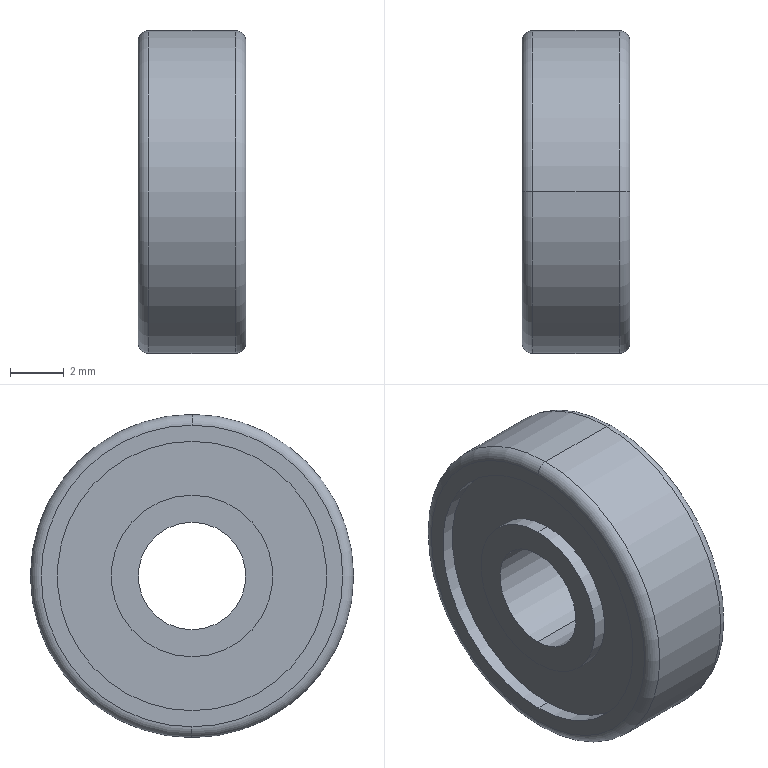Part | STEP file | 604 bearing | 1 solid | 22 faces | box 4 x 12 x 12 mm | volume 349.308 mm3 | cylinder 12 | plane 6 | torus 4 | commonest cylinder face diameters 6 x4 10 x4 4 x2 12 x2
STEP:
#1=CARTESIAN_POINT('',(0.,0.,0.));
#2=DIRECTION('',(0.,0.,1.));
#3=DIRECTION('',(1.,0.,0.));
#4=AXIS2_PLACEMENT_3D('',#1,#2,#3);
#5=CARTESIAN_POINT('',(-1.6,0.,-6.));
#6=VERTEX_POINT('',#5);
#7=CARTESIAN_POINT('',(-1.6,0.,6.));
#8=VERTEX_POINT('',#7);
#9=CARTESIAN_POINT('',(-1.6,0.,0.));
#10=DIRECTION('',(1.,0.,0.));
#11=DIRECTION('',(0.,0.,1.));
#12=AXIS2_PLACEMENT_3D('',#9,#10,#11);
#13=CIRCLE('',#12,6.);
#14=CARTESIAN_POINT('',(-1.6,0.,0.));
#15=DIRECTION('',(-1.,0.,0.));
#16=DIRECTION('',(0.,0.,1.));
#17=AXIS2_PLACEMENT_3D('',#14,#15,#16);
#18=TOROIDAL_SURFACE('',#17,5.6,0.4);
#19=CARTESIAN_POINT('',(6.283,0.));
#20=DIRECTION('',(-1.,0.));
#21=VECTOR('',#20,1.);
#22=LINE('',#19,#21);
#23=(GEOMETRIC_REPRESENTATION_CONTEXT(2)PARAMETRIC_REPRESENTATION_CONTEXT()REPRESENTATION_CONTEXT('',''));
#24=DEFINITIONAL_REPRESENTATION('',(#22),#23);
#25=PCURVE('',#18,#24);
#26=CARTESIAN_POINT('',(0.,0.,0.));
#27=DIRECTION('',(1.,0.,0.));
#28=DIRECTION('',(0.,0.,-1.));
#29=AXIS2_PLACEMENT_3D('',#26,#27,#28);
#30=CYLINDRICAL_SURFACE('',#29,6.);
#31=CARTESIAN_POINT('',(-3.142,-1.6));
#32=DIRECTION('',(1.,0.));
#33=VECTOR('',#32,1.);
#34=LINE('',#31,#33);
#35=(GEOMETRIC_REPRESENTATION_CONTEXT(2)PARAMETRIC_REPRESENTATION_CONTEXT()REPRESENTATION_CONTEXT('',''));
#36=DEFINITIONAL_REPRESENTATION('',(#34),#35);
#37=PCURVE('',#30,#36);
#38=SURFACE_CURVE('',#13,(#25,#37),.PCURVE_S1.);
#39=EDGE_CURVE('',#6,#8,#38,.T.);
#40=ORIENTED_EDGE('',*,*,#39,.F.);
#41=CARTESIAN_POINT('',(-2.,0.,-5.6));
#42=VERTEX_POINT('',#41);
#43=CARTESIAN_POINT('',(-1.6,0.,-5.6));
#44=DIRECTION('',(0.,1.,0.));
#45=DIRECTION('',(0.,0.,1.));
#46=AXIS2_PLACEMENT_3D('',#43,#44,#45);
#47=CIRCLE('',#46,0.4);
#48=CARTESIAN_POINT('',(3.142,-3.142));
#49=DIRECTION('',(0.,1.));
#50=VECTOR('',#49,1.);
#51=LINE('',#48,#50);
#52=(GEOMETRIC_REPRESENTATION_CONTEXT(2)PARAMETRIC_REPRESENTATION_CONTEXT()REPRESENTATION_CONTEXT('',''));
#53=DEFINITIONAL_REPRESENTATION('',(#51),#52);
#54=PCURVE('',#18,#53);
#55=CARTESIAN_POINT('',(-1.6,0.,0.));
#56=DIRECTION('',(-1.,0.,0.));
#57=DIRECTION('',(0.,0.,1.));
#58=AXIS2_PLACEMENT_3D('',#55,#56,#57);
#59=TOROIDAL_SURFACE('',#58,5.6,0.4);
#60=CARTESIAN_POINT('',(3.142,-3.142));
#61=DIRECTION('',(0.,1.));
#62=VECTOR('',#61,1.);
#63=LINE('',#60,#62);
#64=(GEOMETRIC_REPRESENTATION_CONTEXT(2)PARAMETRIC_REPRESENTATION_CONTEXT()REPRESENTATION_CONTEXT('',''));
#65=DEFINITIONAL_REPRESENTATION('',(#63),#64);
#66=PCURVE('',#59,#65);
#67=SURFACE_CURVE('',#47,(#54,#66),.PCURVE_S1.);
#68=EDGE_CURVE('',#6,#42,#67,.T.);
#69=ORIENTED_EDGE('',*,*,#68,.T.);
#70=CARTESIAN_POINT('',(-2.,0.,5.6));
#71=VERTEX_POINT('',#70);
#72=CARTESIAN_POINT('',(-2.,0.,0.));
#73=DIRECTION('',(-1.,0.,0.));
#74=DIRECTION('',(0.,0.,1.));
#75=AXIS2_PLACEMENT_3D('',#72,#73,#74);
#76=CIRCLE('',#75,5.6);
#77=CARTESIAN_POINT('',(0.,1.571));
#78=DIRECTION('',(1.,0.));
#79=VECTOR('',#78,1.);
#80=LINE('',#77,#79);
#81=(GEOMETRIC_REPRESENTATION_CONTEXT(2)PARAMETRIC_REPRESENTATION_CONTEXT()REPRESENTATION_CONTEXT('',''));
#82=DEFINITIONAL_REPRESENTATION('',(#80),#81);
#83=PCURVE('',#18,#82);
#84=CARTESIAN_POINT('',(-2.,6.,0.));
#85=DIRECTION('',(-1.,0.,0.));
#86=DIRECTION('',(0.,0.,1.));
#87=AXIS2_PLACEMENT_3D('',#84,#85,#86);
#88=PLANE('',#87);
#89=CARTESIAN_POINT('',(0.,-6.));
#90=DIRECTION('',(1.,0.));
#91=AXIS2_PLACEMENT_2D('',#89,#90);
#92=CIRCLE('',#91,5.6);
#93=(GEOMETRIC_REPRESENTATION_CONTEXT(2)PARAMETRIC_REPRESENTATION_CONTEXT()REPRESENTATION_CONTEXT('',''));
#94=DEFINITIONAL_REPRESENTATION('',(#92),#93);
#95=PCURVE('',#88,#94);
#96=SURFACE_CURVE('',#76,(#83,#95),.PCURVE_S1.);
#97=EDGE_CURVE('',#71,#42,#96,.T.);
#98=ORIENTED_EDGE('',*,*,#97,.F.);
#99=CARTESIAN_POINT('',(-1.6,0.,5.6));
#100=DIRECTION('',(0.,-1.,0.));
#101=DIRECTION('',(0.,0.,-1.));
#102=AXIS2_PLACEMENT_3D('',#99,#100,#101);
#103=CIRCLE('',#102,0.4);
#104=CARTESIAN_POINT('',(0.,-3.142));
#105=DIRECTION('',(0.,1.));
#106=VECTOR('',#105,1.);
#107=LINE('',#104,#106);
#108=(GEOMETRIC_REPRESENTATION_CONTEXT(2)PARAMETRIC_REPRESENTATION_CONTEXT()REPRESENTATION_CONTEXT('',''));
#109=DEFINITIONAL_REPRESENTATION('',(#107),#108);
#110=PCURVE('',#18,#109);
#111=CARTESIAN_POINT('',(6.283,-3.142));
#112=DIRECTION('',(0.,1.));
#113=VECTOR('',#112,1.);
#114=LINE('',#111,#113);
#115=(GEOMETRIC_REPRESENTATION_CONTEXT(2)PARAMETRIC_REPRESENTATION_CONTEXT()REPRESENTATION_CONTEXT('',''));
#116=DEFINITIONAL_REPRESENTATION('',(#114),#115);
#117=PCURVE('',#59,#116);
#118=SURFACE_CURVE('',#103,(#110,#117),.PCURVE_S1.);
#119=EDGE_CURVE('',#8,#71,#118,.T.);
#120=ORIENTED_EDGE('',*,*,#119,.F.);
#121=EDGE_LOOP('',(#40,#69,#98,#120));
#122=FACE_BOUND('',#121,.T.);
#123=ADVANCED_FACE('',(#122),#18,.T.);
#124=CARTESIAN_POINT('',(1.6,0.,6.));
#125=VERTEX_POINT('',#124);
#126=CARTESIAN_POINT('',(1.6,0.,-6.));
#127=VERTEX_POINT('',#126);
#128=CARTESIAN_POINT('',(1.6,0.,0.));
#129=DIRECTION('',(-1.,0.,0.));
#130=DIRECTION('',(0.,0.,-1.));
#131=AXIS2_PLACEMENT_3D('',#128,#129,#130);
#132=CIRCLE('',#131,6.);
#133=CARTESIAN_POINT('',(1.6,0.,0.));
#134=DIRECTION('',(1.,0.,0.));
#135=DIRECTION('',(0.,0.,-1.));
#136=AXIS2_PLACEMENT_3D('',#133,#134,#135);
#137=TOROIDAL_SURFACE('',#136,5.6,0.4);
#138=CARTESIAN_POINT('',(6.283,0.));
#139=DIRECTION('',(-1.,0.));
#140=VECTOR('',#139,1.);
#141=LINE('',#138,#140);
#142=(GEOMETRIC_REPRESENTATION_CONTEXT(2)PARAMETRIC_REPRESENTATION_CONTEXT()REPRESENTATION_CONTEXT('',''));
#143=DEFINITIONAL_REPRESENTATION('',(#141),#142);
#144=PCURVE('',#137,#143);
#145=CARTESIAN_POINT('',(6.283,1.6));
#146=DIRECTION('',(-1.,0.));
#147=VECTOR('',#146,1.);
#148=LINE('',#145,#147);
#149=(GEOMETRIC_REPRESENTATION_CONTEXT(2)PARAMETRIC_REPRESENTATION_CONTEXT()REPRESENTATION_CONTEXT('',''));
#150=DEFINITIONAL_REPRESENTATION('',(#148),#149);
#151=PCURVE('',#30,#150);
#152=SURFACE_CURVE('',#132,(#144,#151),.PCURVE_S1.);
#153=EDGE_CURVE('',#125,#127,#152,.T.);
#154=ORIENTED_EDGE('',*,*,#153,.F.);
#155=CARTESIAN_POINT('',(2.,0.,5.6));
#156=VERTEX_POINT('',#155);
#157=CARTESIAN_POINT('',(1.6,0.,5.6));
#158=DIRECTION('',(0.,1.,0.));
#159=DIRECTION('',(0.,0.,1.));
#160=AXIS2_PLACEMENT_3D('',#157,#158,#159);
#161=CIRCLE('',#160,0.4);
#162=CARTESIAN_POINT('',(3.142,0.));
#163=DIRECTION('',(0.,1.));
#164=VECTOR('',#163,1.);
#165=LINE('',#162,#164);
#166=(GEOMETRIC_REPRESENTATION_CONTEXT(2)PARAMETRIC_REPRESENTATION_CONTEXT()REPRESENTATION_CONTEXT('',''));
#167=DEFINITIONAL_REPRESENTATION('',(#165),#166);
#168=PCURVE('',#137,#167);
#169=CARTESIAN_POINT('',(1.6,0.,0.));
#170=DIRECTION('',(1.,0.,0.));
#171=DIRECTION('',(0.,0.,-1.));
#172=AXIS2_PLACEMENT_3D('',#169,#170,#171);
#173=TOROIDAL_SURFACE('',#172,5.6,0.4);
#174=CARTESIAN_POINT('',(3.142,0.));
#175=DIRECTION('',(0.,1.));
#176=VECTOR('',#175,1.);
#177=LINE('',#174,#176);
#178=(GEOMETRIC_REPRESENTATION_CONTEXT(2)PARAMETRIC_REPRESENTATION_CONTEXT()REPRESENTATION_CONTEXT('',''));
#179=DEFINITIONAL_REPRESENTATION('',(#177),#178);
#180=PCURVE('',#173,#179);
#181=SURFACE_CURVE('',#161,(#168,#180),.PCURVE_S1.);
#182=EDGE_CURVE('',#125,#156,#181,.T.);
#183=ORIENTED_EDGE('',*,*,#182,.T.);
#184=CARTESIAN_POINT('',(2.,0.,-5.6));
#185=VERTEX_POINT('',#184);
#186=CARTESIAN_POINT('',(2.,0.,0.));
#187=DIRECTION('',(1.,0.,0.));
#188=DIRECTION('',(0.,0.,-1.));
#189=AXIS2_PLACEMENT_3D('',#186,#187,#188);
#190=CIRCLE('',#189,5.6);
#191=CARTESIAN_POINT('',(0.,1.571));
#192=DIRECTION('',(1.,0.));
#193=VECTOR('',#192,1.);
#194=LINE('',#191,#193);
#195=(GEOMETRIC_REPRESENTATION_CONTEXT(2)PARAMETRIC_REPRESENTATION_CONTEXT()REPRESENTATION_CONTEXT('',''));
#196=DEFINITIONAL_REPRESENTATION('',(#194),#195);
#197=PCURVE('',#137,#196);
#198=CARTESIAN_POINT('',(2.,6.,0.));
#199=DIRECTION('',(1.,0.,0.));
#200=DIRECTION('',(0.,0.,-1.));
#201=AXIS2_PLACEMENT_3D('',#198,#199,#200);
#202=PLANE('',#201);
#203=CARTESIAN_POINT('',(0.,-6.));
#204=DIRECTION('',(1.,0.));
#205=AXIS2_PLACEMENT_2D('',#203,#204);
#206=CIRCLE('',#205,5.6);
#207=(GEOMETRIC_REPRESENTATION_CONTEXT(2)PARAMETRIC_REPRESENTATION_CONTEXT()REPRESENTATION_CONTEXT('',''));
#208=DEFINITIONAL_REPRESENTATION('',(#206),#207);
#209=PCURVE('',#202,#208);
#210=SURFACE_CURVE('',#190,(#197,#209),.PCURVE_S1.);
#211=EDGE_CURVE('',#185,#156,#210,.T.);
#212=ORIENTED_EDGE('',*,*,#211,.F.);
#213=CARTESIAN_POINT('',(1.6,0.,-5.6));
#214=DIRECTION('',(0.,-1.,0.));
#215=DIRECTION('',(0.,0.,-1.));
#216=AXIS2_PLACEMENT_3D('',#213,#214,#215);
#217=CIRCLE('',#216,0.4);
#218=CARTESIAN_POINT('',(0.,0.));
#219=DIRECTION('',(0.,1.));
#220=VECTOR('',#219,1.);
#221=LINE('',#218,#220);
#222=(GEOMETRIC_REPRESENTATION_CONTEXT(2)PARAMETRIC_REPRESENTATION_CONTEXT()REPRESENTATION_CONTEXT('',''));
#223=DEFINITIONAL_REPRESENTATION('',(#221),#222);
#224=PCURVE('',#137,#223);
#225=CARTESIAN_POINT('',(6.283,0.));
#226=DIRECTION('',(0.,1.));
#227=VECTOR('',#226,1.);
#228=LINE('',#225,#227);
#229=(GEOMETRIC_REPRESENTATION_CONTEXT(2)PARAMETRIC_REPRESENTATION_CONTEXT()REPRESENTATION_CONTEXT('',''));
#230=DEFINITIONAL_REPRESENTATION('',(#228),#229);
#231=PCURVE('',#173,#230);
#232=SURFACE_CURVE('',#217,(#224,#231),.PCURVE_S1.);
#233=EDGE_CURVE('',#127,#185,#232,.T.);
#234=ORIENTED_EDGE('',*,*,#233,.F.);
#235=EDGE_LOOP('',(#154,#183,#212,#234));
#236=FACE_BOUND('',#235,.T.);
#237=ADVANCED_FACE('',(#236),#137,.T.);
#238=CARTESIAN_POINT('',(1.5,0.,3.));
#239=VERTEX_POINT('',#238);
#240=CARTESIAN_POINT('',(1.5,0.,-3.));
#241=VERTEX_POINT('',#240);
#242=CARTESIAN_POINT('',(1.5,0.,0.));
#243=DIRECTION('',(-1.,0.,0.));
#244=DIRECTION('',(0.,0.,1.));
#245=AXIS2_PLACEMENT_3D('',#242,#243,#244);
#246=CIRCLE('',#245,3.);
#247=CARTESIAN_POINT('',(1.5,0.,0.));
#248=DIRECTION('',(1.,0.,0.));
#249=DIRECTION('',(0.,0.,-1.));
#250=AXIS2_PLACEMENT_3D('',#247,#248,#249);
#251=CYLINDRICAL_SURFACE('',#250,3.);
#252=CARTESIAN_POINT('',(3.142,0.));
#253=DIRECTION('',(-1.,0.));
#254=VECTOR('',#253,1.);
#255=LINE('',#252,#254);
#256=(GEOMETRIC_REPRESENTATION_CONTEXT(2)PARAMETRIC_REPRESENTATION_CONTEXT()REPRESENTATION_CONTEXT('',''));
#257=DEFINITIONAL_REPRESENTATION('',(#255),#256);
#258=PCURVE('',#251,#257);
#259=CARTESIAN_POINT('',(1.5,0.,0.));
#260=DIRECTION('',(1.,0.,0.));
#261=DIRECTION('',(0.,0.,1.));
#262=AXIS2_PLACEMENT_3D('',#259,#260,#261);
#263=PLANE('',#262);
#264=CARTESIAN_POINT('',(3.,0.));
#265=CARTESIAN_POINT('',(3.,-5.196));
#266=CARTESIAN_POINT('',(-1.5,-2.598));
#267=CARTESIAN_POINT('',(-6.,0.));
#268=CARTESIAN_POINT('',(-1.5,2.598));
#269=CARTESIAN_POINT('',(3.,5.196));
#270=CARTESIAN_POINT('',(3.,0.));
#271=(BOUNDED_CURVE()B_SPLINE_CURVE(2,(#264,#265,#266,#267,#268,#269,#270),.UNSPECIFIED.,.T.,.F.)B_SPLINE_CURVE_WITH_KNOTS((1,2,2,2,2,1),(-2.094,0.,2.094,4.189,6.283,8.378),.UNSPECIFIED.)CURVE()GEOMETRIC_REPRESENTATION_ITEM()RATIONAL_B_SPLINE_CURVE((1.,0.5,1.,0.5,1.,0.5,1.))REPRESENTATION_ITEM(''));
#272=(GEOMETRIC_REPRESENTATION_CONTEXT(2)PARAMETRIC_REPRESENTATION_CONTEXT()REPRESENTATION_CONTEXT('',''));
#273=DEFINITIONAL_REPRESENTATION('',(#271),#272);
#274=PCURVE('',#263,#273);
#275=SURFACE_CURVE('',#246,(#258,#274),.PCURVE_S1.);
#276=EDGE_CURVE('',#239,#241,#275,.T.);
#277=ORIENTED_EDGE('',*,*,#276,.F.);
#278=CARTESIAN_POINT('',(2.,0.,3.));
#279=VERTEX_POINT('',#278);
#280=CARTESIAN_POINT('',(1.5,0.,3.));
#281=DIRECTION('',(1.,0.,0.));
#282=VECTOR('',#281,1.);
#283=LINE('',#280,#282);
#284=CARTESIAN_POINT('',(3.142,0.));
#285=DIRECTION('',(0.,1.));
#286=VECTOR('',#285,1.);
#287=LINE('',#284,#286);
#288=(GEOMETRIC_REPRESENTATION_CONTEXT(2)PARAMETRIC_REPRESENTATION_CONTEXT()REPRESENTATION_CONTEXT('',''));
#289=DEFINITIONAL_REPRESENTATION('',(#287),#288);
#290=PCURVE('',#251,#289);
#291=CARTESIAN_POINT('',(1.5,0.,0.));
#292=DIRECTION('',(1.,0.,0.));
#293=DIRECTION('',(0.,0.,-1.));
#294=AXIS2_PLACEMENT_3D('',#291,#292,#293);
#295=CYLINDRICAL_SURFACE('',#294,3.);
#296=CARTESIAN_POINT('',(3.142,0.));
#297=DIRECTION('',(0.,1.));
#298=VECTOR('',#297,1.);
#299=LINE('',#296,#298);
#300=(GEOMETRIC_REPRESENTATION_CONTEXT(2)PARAMETRIC_REPRESENTATION_CONTEXT()REPRESENTATION_CONTEXT('',''));
#301=DEFINITIONAL_REPRESENTATION('',(#299),#300);
#302=PCURVE('',#295,#301);
#303=SURFACE_CURVE('',#283,(#290,#302),.PCURVE_S1.);
#304=EDGE_CURVE('',#239,#279,#303,.T.);
#305=ORIENTED_EDGE('',*,*,#304,.T.);
#306=CARTESIAN_POINT('',(2.,0.,-3.));
#307=VERTEX_POINT('',#306);
#308=CARTESIAN_POINT('',(2.,0.,0.));
#309=DIRECTION('',(-1.,0.,0.));
#310=DIRECTION('',(0.,0.,1.));
#311=AXIS2_PLACEMENT_3D('',#308,#309,#310);
#312=CIRCLE('',#311,3.);
#313=CARTESIAN_POINT('',(3.142,0.5));
#314=DIRECTION('',(-1.,0.));
#315=VECTOR('',#314,1.);
#316=LINE('',#313,#315);
#317=(GEOMETRIC_REPRESENTATION_CONTEXT(2)PARAMETRIC_REPRESENTATION_CONTEXT()REPRESENTATION_CONTEXT('',''));
#318=DEFINITIONAL_REPRESENTATION('',(#316),#317);
#319=PCURVE('',#251,#318);
#320=CARTESIAN_POINT('',(2.,6.,0.));
#321=DIRECTION('',(1.,0.,0.));
#322=DIRECTION('',(0.,0.,-1.));
#323=AXIS2_PLACEMENT_3D('',#320,#321,#322);
#324=PLANE('',#323);
#325=CARTESIAN_POINT('',(-3.,-6.));
#326=CARTESIAN_POINT('',(-3.,-0.8038));
#327=CARTESIAN_POINT('',(1.5,-3.402));
#328=CARTESIAN_POINT('',(6.,-6.));
#329=CARTESIAN_POINT('',(1.5,-8.598));
#330=CARTESIAN_POINT('',(-3.,-11.196));
#331=CARTESIAN_POINT('',(-3.,-6.));
#332=(BOUNDED_CURVE()B_SPLINE_CURVE(2,(#325,#326,#327,#328,#329,#330,#331),.UNSPECIFIED.,.T.,.F.)B_SPLINE_CURVE_WITH_KNOTS((1,2,2,2,2,1),(-2.094,0.,2.094,4.189,6.283,8.378),.UNSPECIFIED.)CURVE()GEOMETRIC_REPRESENTATION_ITEM()RATIONAL_B_SPLINE_CURVE((1.,0.5,1.,0.5,1.,0.5,1.))REPRESENTATION_ITEM(''));
#333=(GEOMETRIC_REPRESENTATION_CONTEXT(2)PARAMETRIC_REPRESENTATION_CONTEXT()REPRESENTATION_CONTEXT('',''));
#334=DEFINITIONAL_REPRESENTATION('',(#332),#333);
#335=PCURVE('',#324,#334);
#336=SURFACE_CURVE('',#312,(#319,#335),.PCURVE_S1.);
#337=EDGE_CURVE('',#279,#307,#336,.T.);
#338=ORIENTED_EDGE('',*,*,#337,.T.);
#339=CARTESIAN_POINT('',(1.5,0.,-3.));
#340=DIRECTION('',(1.,0.,0.));
#341=VECTOR('',#340,1.);
#342=LINE('',#339,#341);
#343=CARTESIAN_POINT('',(0.,0.));
#344=DIRECTION('',(0.,1.));
#345=VECTOR('',#344,1.);
#346=LINE('',#343,#345);
#347=(GEOMETRIC_REPRESENTATION_CONTEXT(2)PARAMETRIC_REPRESENTATION_CONTEXT()REPRESENTATION_CONTEXT('',''));
#348=DEFINITIONAL_REPRESENTATION('',(#346),#347);
#349=PCURVE('',#251,#348);
#350=CARTESIAN_POINT('',(6.283,0.));
#351=DIRECTION('',(0.,1.));
#352=VECTOR('',#351,1.);
#353=LINE('',#350,#352);
#354=(GEOMETRIC_REPRESENTATION_CONTEXT(2)PARAMETRIC_REPRESENTATION_CONTEXT()REPRESENTATION_CONTEXT('',''));
#355=DEFINITIONAL_REPRESENTATION('',(#353),#354);
#356=PCURVE('',#295,#355);
#357=SURFACE_CURVE('',#342,(#349,#356),.PCURVE_S1.);
#358=EDGE_CURVE('',#241,#307,#357,.T.);
#359=ORIENTED_EDGE('',*,*,#358,.F.);
#360=EDGE_LOOP('',(#277,#305,#338,#359));
#361=FACE_BOUND('',#360,.T.);
#362=ADVANCED_FACE('',(#361),#251,.T.);
#363=CARTESIAN_POINT('',(1.5,0.,-5.));
#364=VERTEX_POINT('',#363);
#365=CARTESIAN_POINT('',(2.,0.,-5.));
#366=VERTEX_POINT('',#365);
#367=CARTESIAN_POINT('',(1.5,0.,-5.));
#368=DIRECTION('',(1.,0.,0.));
#369=VECTOR('',#368,1.);
#370=LINE('',#367,#369);
#371=CARTESIAN_POINT('',(1.5,0.,0.));
#372=DIRECTION('',(1.,0.,0.));
#373=DIRECTION('',(0.,0.,-1.));
#374=AXIS2_PLACEMENT_3D('',#371,#372,#373);
#375=CYLINDRICAL_SURFACE('',#374,5.);
#376=CARTESIAN_POINT('',(6.283,0.));
#377=DIRECTION('',(0.,1.));
#378=VECTOR('',#377,1.);
#379=LINE('',#376,#378);
#380=(GEOMETRIC_REPRESENTATION_CONTEXT(2)PARAMETRIC_REPRESENTATION_CONTEXT()REPRESENTATION_CONTEXT('',''));
#381=DEFINITIONAL_REPRESENTATION('',(#379),#380);
#382=PCURVE('',#375,#381);
#383=CARTESIAN_POINT('',(1.5,0.,0.));
#384=DIRECTION('',(1.,0.,0.));
#385=DIRECTION('',(0.,0.,-1.));
#386=AXIS2_PLACEMENT_3D('',#383,#384,#385);
#387=CYLINDRICAL_SURFACE('',#386,5.);
#388=CARTESIAN_POINT('',(0.,0.));
#389=DIRECTION('',(0.,1.));
#390=VECTOR('',#389,1.);
#391=LINE('',#388,#390);
#392=(GEOMETRIC_REPRESENTATION_CONTEXT(2)PARAMETRIC_REPRESENTATION_CONTEXT()REPRESENTATION_CONTEXT('',''));
#393=DEFINITIONAL_REPRESENTATION('',(#391),#392);
#394=PCURVE('',#387,#393);
#395=SURFACE_CURVE('',#370,(#382,#394),.PCURVE_S1.);
#396=EDGE_CURVE('',#364,#366,#395,.T.);
#397=ORIENTED_EDGE('',*,*,#396,.T.);
#398=CARTESIAN_POINT('',(2.,0.,5.));
#399=VERTEX_POINT('',#398);
#400=CARTESIAN_POINT('',(2.,0.,0.));
#401=DIRECTION('',(-1.,0.,0.));
#402=DIRECTION('',(0.,0.,1.));
#403=AXIS2_PLACEMENT_3D('',#400,#401,#402);
#404=CIRCLE('',#403,5.);
#405=CARTESIAN_POINT('',(9.425,0.5));
#406=DIRECTION('',(-1.,0.));
#407=VECTOR('',#406,1.);
#408=LINE('',#405,#407);
#409=(GEOMETRIC_REPRESENTATION_CONTEXT(2)PARAMETRIC_REPRESENTATION_CONTEXT()REPRESENTATION_CONTEXT('',''));
#410=DEFINITIONAL_REPRESENTATION('',(#408),#409);
#411=PCURVE('',#375,#410);
#412=CARTESIAN_POINT('',(-5.,-6.));
#413=CARTESIAN_POINT('',(-5.,2.66));
#414=CARTESIAN_POINT('',(2.5,-1.67));
#415=CARTESIAN_POINT('',(10.,-6.));
#416=CARTESIAN_POINT('',(2.5,-10.33));
#417=CARTESIAN_POINT('',(-5.,-14.66));
#418=CARTESIAN_POINT('',(-5.,-6.));
#419=(BOUNDED_CURVE()B_SPLINE_CURVE(2,(#412,#413,#414,#415,#416,#417,#418),.UNSPECIFIED.,.T.,.F.)B_SPLINE_CURVE_WITH_KNOTS((1,2,2,2,2,1),(-2.094,0.,2.094,4.189,6.283,8.378),.UNSPECIFIED.)CURVE()GEOMETRIC_REPRESENTATION_ITEM()RATIONAL_B_SPLINE_CURVE((1.,0.5,1.,0.5,1.,0.5,1.))REPRESENTATION_ITEM(''));
#420=(GEOMETRIC_REPRESENTATION_CONTEXT(2)PARAMETRIC_REPRESENTATION_CONTEXT()REPRESENTATION_CONTEXT('',''));
#421=DEFINITIONAL_REPRESENTATION('',(#419),#420);
#422=PCURVE('',#202,#421);
#423=SURFACE_CURVE('',#404,(#411,#422),.PCURVE_S1.);
#424=EDGE_CURVE('',#366,#399,#423,.T.);
#425=ORIENTED_EDGE('',*,*,#424,.T.);
#426=CARTESIAN_POINT('',(1.5,0.,5.));
#427=VERTEX_POINT('',#426);
#428=CARTESIAN_POINT('',(1.5,0.,5.));
#429=DIRECTION('',(1.,0.,0.));
#430=VECTOR('',#429,1.);
#431=LINE('',#428,#430);
#432=CARTESIAN_POINT('',(3.142,0.));
#433=DIRECTION('',(0.,1.));
#434=VECTOR('',#433,1.);
#435=LINE('',#432,#434);
#436=(GEOMETRIC_REPRESENTATION_CONTEXT(2)PARAMETRIC_REPRESENTATION_CONTEXT()REPRESENTATION_CONTEXT('',''));
#437=DEFINITIONAL_REPRESENTATION('',(#435),#436);
#438=PCURVE('',#375,#437);
#439=CARTESIAN_POINT('',(3.142,0.));
#440=DIRECTION('',(0.,1.));
#441=VECTOR('',#440,1.);
#442=LINE('',#439,#441);
#443=(GEOMETRIC_REPRESENTATION_CONTEXT(2)PARAMETRIC_REPRESENTATION_CONTEXT()REPRESENTATION_CONTEXT('',''));
#444=DEFINITIONAL_REPRESENTATION('',(#442),#443);
#445=PCURVE('',#387,#444);
#446=SURFACE_CURVE('',#431,(#438,#445),.PCURVE_S1.);
#447=EDGE_CURVE('',#427,#399,#446,.T.);
#448=ORIENTED_EDGE('',*,*,#447,.F.);
#449=CARTESIAN_POINT('',(1.5,0.,0.));
#450=DIRECTION('',(-1.,0.,0.));
#451=DIRECTION('',(0.,0.,1.));
#452=AXIS2_PLACEMENT_3D('',#449,#450,#451);
#453=CIRCLE('',#452,5.);
#454=CARTESIAN_POINT('',(9.425,0.));
#455=DIRECTION('',(-1.,0.));
#456=VECTOR('',#455,1.);
#457=LINE('',#454,#456);
#458=(GEOMETRIC_REPRESENTATION_CONTEXT(2)PARAMETRIC_REPRESENTATION_CONTEXT()REPRESENTATION_CONTEXT('',''));
#459=DEFINITIONAL_REPRESENTATION('',(#457),#458);
#460=PCURVE('',#375,#459);
#461=CARTESIAN_POINT('',(5.,0.));
#462=CARTESIAN_POINT('',(5.,-8.66));
#463=CARTESIAN_POINT('',(-2.5,-4.33));
#464=CARTESIAN_POINT('',(-10.,0.));
#465=CARTESIAN_POINT('',(-2.5,4.33));
#466=CARTESIAN_POINT('',(5.,8.66));
#467=CARTESIAN_POINT('',(5.,0.));
#468=(BOUNDED_CURVE()B_SPLINE_CURVE(2,(#461,#462,#463,#464,#465,#466,#467),.UNSPECIFIED.,.T.,.F.)B_SPLINE_CURVE_WITH_KNOTS((1,2,2,2,2,1),(-2.094,0.,2.094,4.189,6.283,8.378),.UNSPECIFIED.)CURVE()GEOMETRIC_REPRESENTATION_ITEM()RATIONAL_B_SPLINE_CURVE((1.,0.5,1.,0.5,1.,0.5,1.))REPRESENTATION_ITEM(''));
#469=(GEOMETRIC_REPRESENTATION_CONTEXT(2)PARAMETRIC_REPRESENTATION_CONTEXT()REPRESENTATION_CONTEXT('',''));
#470=DEFINITIONAL_REPRESENTATION('',(#468),#469);
#471=PCURVE('',#263,#470);
#472=SURFACE_CURVE('',#453,(#460,#471),.PCURVE_S1.);
#473=EDGE_CURVE('',#364,#427,#472,.T.);
#474=ORIENTED_EDGE('',*,*,#473,.F.);
#475=EDGE_LOOP('',(#397,#425,#448,#474));
#476=FACE_BOUND('',#475,.F.);
#477=ADVANCED_FACE('',(#476),#375,.F.);
#478=CARTESIAN_POINT('',(-1.5,0.,3.));
#479=VERTEX_POINT('',#478);
#480=CARTESIAN_POINT('',(-1.5,0.,-3.));
#481=VERTEX_POINT('',#480);
#482=CARTESIAN_POINT('',(-1.5,0.,0.));
#483=DIRECTION('',(-1.,0.,0.));
#484=DIRECTION('',(0.,0.,1.));
#485=AXIS2_PLACEMENT_3D('',#482,#483,#484);
#486=CIRCLE('',#485,3.);
#487=CARTESIAN_POINT('',(-1.5,0.,0.));
#488=DIRECTION('',(-1.,0.,0.));
#489=DIRECTION('',(0.,0.,1.));
#490=AXIS2_PLACEMENT_3D('',#487,#488,#489);
#491=CYLINDRICAL_SURFACE('',#490,3.);
#492=CARTESIAN_POINT('',(0.,0.));
#493=DIRECTION('',(1.,0.));
#494=VECTOR('',#493,1.);
#495=LINE('',#492,#494);
#496=(GEOMETRIC_REPRESENTATION_CONTEXT(2)PARAMETRIC_REPRESENTATION_CONTEXT()REPRESENTATION_CONTEXT('',''));
#497=DEFINITIONAL_REPRESENTATION('',(#495),#496);
#498=PCURVE('',#491,#497);
#499=CARTESIAN_POINT('',(-1.5,0.,0.));
#500=DIRECTION('',(-1.,0.,0.));
#501=DIRECTION('',(0.,0.,1.));
#502=AXIS2_PLACEMENT_3D('',#499,#500,#501);
#503=PLANE('',#502);
#504=CARTESIAN_POINT('',(0.,0.));
#505=DIRECTION('',(1.,0.));
#506=AXIS2_PLACEMENT_2D('',#504,#505);
#507=CIRCLE('',#506,3.);
#508=(GEOMETRIC_REPRESENTATION_CONTEXT(2)PARAMETRIC_REPRESENTATION_CONTEXT()REPRESENTATION_CONTEXT('',''));
#509=DEFINITIONAL_REPRESENTATION('',(#507),#508);
#510=PCURVE('',#503,#509);
#511=SURFACE_CURVE('',#486,(#498,#510),.PCURVE_S1.);
#512=EDGE_CURVE('',#479,#481,#511,.T.);
#513=ORIENTED_EDGE('',*,*,#512,.T.);
#514=CARTESIAN_POINT('',(-2.,0.,-3.));
#515=VERTEX_POINT('',#514);
#516=CARTESIAN_POINT('',(-1.5,0.,-3.));
#517=DIRECTION('',(-1.,0.,0.));
#518=VECTOR('',#517,1.);
#519=LINE('',#516,#518);
#520=CARTESIAN_POINT('',(3.142,0.));
#521=DIRECTION('',(0.,1.));
#522=VECTOR('',#521,1.);
#523=LINE('',#520,#522);
#524=(GEOMETRIC_REPRESENTATION_CONTEXT(2)PARAMETRIC_REPRESENTATION_CONTEXT()REPRESENTATION_CONTEXT('',''));
#525=DEFINITIONAL_REPRESENTATION('',(#523),#524);
#526=PCURVE('',#491,#525);
#527=CARTESIAN_POINT('',(-1.5,0.,0.));
#528=DIRECTION('',(-1.,0.,0.));
#529=DIRECTION('',(0.,0.,1.));
#530=AXIS2_PLACEMENT_3D('',#527,#528,#529);
#531=CYLINDRICAL_SURFACE('',#530,3.);
#532=CARTESIAN_POINT('',(3.142,0.));
#533=DIRECTION('',(0.,1.));
#534=VECTOR('',#533,1.);
#535=LINE('',#532,#534);
#536=(GEOMETRIC_REPRESENTATION_CONTEXT(2)PARAMETRIC_REPRESENTATION_CONTEXT()REPRESENTATION_CONTEXT('',''));
#537=DEFINITIONAL_REPRESENTATION('',(#535),#536);
#538=PCURVE('',#531,#537);
#539=SURFACE_CURVE('',#519,(#526,#538),.PCURVE_S1.);
#540=EDGE_CURVE('',#481,#515,#539,.T.);
#541=ORIENTED_EDGE('',*,*,#540,.T.);
#542=CARTESIAN_POINT('',(-2.,0.,3.));
#543=VERTEX_POINT('',#542);
#544=CARTESIAN_POINT('',(-2.,0.,0.));
#545=DIRECTION('',(-1.,0.,0.));
#546=DIRECTION('',(0.,0.,1.));
#547=AXIS2_PLACEMENT_3D('',#544,#545,#546);
#548=CIRCLE('',#547,3.);
#549=CARTESIAN_POINT('',(0.,0.5));
#550=DIRECTION('',(1.,0.));
#551=VECTOR('',#550,1.);
#552=LINE('',#549,#551);
#553=(GEOMETRIC_REPRESENTATION_CONTEXT(2)PARAMETRIC_REPRESENTATION_CONTEXT()REPRESENTATION_CONTEXT('',''));
#554=DEFINITIONAL_REPRESENTATION('',(#552),#553);
#555=PCURVE('',#491,#554);
#556=CARTESIAN_POINT('',(-2.,6.,0.));
#557=DIRECTION('',(-1.,0.,0.));
#558=DIRECTION('',(0.,0.,1.));
#559=AXIS2_PLACEMENT_3D('',#556,#557,#558);
#560=PLANE('',#559);
#561=CARTESIAN_POINT('',(0.,-6.));
#562=DIRECTION('',(1.,0.));
#563=AXIS2_PLACEMENT_2D('',#561,#562);
#564=CIRCLE('',#563,3.);
#565=(GEOMETRIC_REPRESENTATION_CONTEXT(2)PARAMETRIC_REPRESENTATION_CONTEXT()REPRESENTATION_CONTEXT('',''));
#566=DEFINITIONAL_REPRESENTATION('',(#564),#565);
#567=PCURVE('',#560,#566);
#568=SURFACE_CURVE('',#548,(#555,#567),.PCURVE_S1.);
#569=EDGE_CURVE('',#543,#515,#568,.T.);
#570=ORIENTED_EDGE('',*,*,#569,.F.);
#571=CARTESIAN_POINT('',(-1.5,0.,3.));
#572=DIRECTION('',(-1.,0.,0.));
#573=VECTOR('',#572,1.);
#574=LINE('',#571,#573);
#575=CARTESIAN_POINT('',(0.,0.));
#576=DIRECTION('',(0.,1.));
#577=VECTOR('',#576,1.);
#578=LINE('',#575,#577);
#579=(GEOMETRIC_REPRESENTATION_CONTEXT(2)PARAMETRIC_REPRESENTATION_CONTEXT()REPRESENTATION_CONTEXT('',''));
#580=DEFINITIONAL_REPRESENTATION('',(#578),#579);
#581=PCURVE('',#491,#580);
#582=CARTESIAN_POINT('',(6.283,0.));
#583=DIRECTION('',(0.,1.));
#584=VECTOR('',#583,1.);
#585=LINE('',#582,#584);
#586=(GEOMETRIC_REPRESENTATION_CONTEXT(2)PARAMETRIC_REPRESENTATION_CONTEXT()REPRESENTATION_CONTEXT('',''));
#587=DEFINITIONAL_REPRESENTATION('',(#585),#586);
#588=PCURVE('',#531,#587);
#589=SURFACE_CURVE('',#574,(#581,#588),.PCURVE_S1.);
#590=EDGE_CURVE('',#479,#543,#589,.T.);
#591=ORIENTED_EDGE('',*,*,#590,.F.);
#592=EDGE_LOOP('',(#513,#541,#570,#591));
#593=FACE_BOUND('',#592,.T.);
#594=ADVANCED_FACE('',(#593),#491,.T.);
#595=CARTESIAN_POINT('',(-1.5,0.,5.));
#596=VERTEX_POINT('',#595);
#597=CARTESIAN_POINT('',(-2.,0.,5.));
#598=VERTEX_POINT('',#597);
#599=CARTESIAN_POINT('',(-1.5,0.,5.));
#600=DIRECTION('',(-1.,0.,0.));
#601=VECTOR('',#600,1.);
#602=LINE('',#599,#601);
#603=CARTESIAN_POINT('',(-1.5,0.,0.));
#604=DIRECTION('',(-1.,0.,0.));
#605=DIRECTION('',(0.,0.,1.));
#606=AXIS2_PLACEMENT_3D('',#603,#604,#605);
#607=CYLINDRICAL_SURFACE('',#606,5.);
#608=CARTESIAN_POINT('',(6.283,0.));
#609=DIRECTION('',(0.,1.));
#610=VECTOR('',#609,1.);
#611=LINE('',#608,#610);
#612=(GEOMETRIC_REPRESENTATION_CONTEXT(2)PARAMETRIC_REPRESENTATION_CONTEXT()REPRESENTATION_CONTEXT('',''));
#613=DEFINITIONAL_REPRESENTATION('',(#611),#612);
#614=PCURVE('',#607,#613);
#615=CARTESIAN_POINT('',(-1.5,0.,0.));
#616=DIRECTION('',(-1.,0.,0.));
#617=DIRECTION('',(0.,0.,1.));
#618=AXIS2_PLACEMENT_3D('',#615,#616,#617);
#619=CYLINDRICAL_SURFACE('',#618,5.);
#620=CARTESIAN_POINT('',(0.,0.));
#621=DIRECTION('',(0.,1.));
#622=VECTOR('',#621,1.);
#623=LINE('',#620,#622);
#624=(GEOMETRIC_REPRESENTATION_CONTEXT(2)PARAMETRIC_REPRESENTATION_CONTEXT()REPRESENTATION_CONTEXT('',''));
#625=DEFINITIONAL_REPRESENTATION('',(#623),#624);
#626=PCURVE('',#619,#625);
#627=SURFACE_CURVE('',#602,(#614,#626),.PCURVE_S1.);
#628=EDGE_CURVE('',#596,#598,#627,.T.);
#629=ORIENTED_EDGE('',*,*,#628,.T.);
#630=CARTESIAN_POINT('',(-2.,0.,-5.));
#631=VERTEX_POINT('',#630);
#632=CARTESIAN_POINT('',(-2.,0.,0.));
#633=DIRECTION('',(-1.,0.,0.));
#634=DIRECTION('',(0.,0.,1.));
#635=AXIS2_PLACEMENT_3D('',#632,#633,#634);
#636=CIRCLE('',#635,5.);
#637=CARTESIAN_POINT('',(0.,0.5));
#638=DIRECTION('',(1.,0.));
#639=VECTOR('',#638,1.);
#640=LINE('',#637,#639);
#641=(GEOMETRIC_REPRESENTATION_CONTEXT(2)PARAMETRIC_REPRESENTATION_CONTEXT()REPRESENTATION_CONTEXT('',''));
#642=DEFINITIONAL_REPRESENTATION('',(#640),#641);
#643=PCURVE('',#607,#642);
#644=CARTESIAN_POINT('',(0.,-6.));
#645=DIRECTION('',(1.,0.));
#646=AXIS2_PLACEMENT_2D('',#644,#645);
#647=CIRCLE('',#646,5.);
#648=(GEOMETRIC_REPRESENTATION_CONTEXT(2)PARAMETRIC_REPRESENTATION_CONTEXT()REPRESENTATION_CONTEXT('',''));
#649=DEFINITIONAL_REPRESENTATION('',(#647),#648);
#650=PCURVE('',#88,#649);
#651=SURFACE_CURVE('',#636,(#643,#650),.PCURVE_S1.);
#652=EDGE_CURVE('',#631,#598,#651,.T.);
#653=ORIENTED_EDGE('',*,*,#652,.F.);
#654=CARTESIAN_POINT('',(-1.5,0.,-5.));
#655=VERTEX_POINT('',#654);
#656=CARTESIAN_POINT('',(-1.5,0.,-5.));
#657=DIRECTION('',(-1.,0.,0.));
#658=VECTOR('',#657,1.);
#659=LINE('',#656,#658);
#660=CARTESIAN_POINT('',(3.142,0.));
#661=DIRECTION('',(0.,1.));
#662=VECTOR('',#661,1.);
#663=LINE('',#660,#662);
#664=(GEOMETRIC_REPRESENTATION_CONTEXT(2)PARAMETRIC_REPRESENTATION_CONTEXT()REPRESENTATION_CONTEXT('',''));
#665=DEFINITIONAL_REPRESENTATION('',(#663),#664);
#666=PCURVE('',#607,#665);
#667=CARTESIAN_POINT('',(3.142,0.));
#668=DIRECTION('',(0.,1.));
#669=VECTOR('',#668,1.);
#670=LINE('',#667,#669);
#671=(GEOMETRIC_REPRESENTATION_CONTEXT(2)PARAMETRIC_REPRESENTATION_CONTEXT()REPRESENTATION_CONTEXT('',''));
#672=DEFINITIONAL_REPRESENTATION('',(#670),#671);
#673=PCURVE('',#619,#672);
#674=SURFACE_CURVE('',#659,(#666,#673),.PCURVE_S1.);
#675=EDGE_CURVE('',#655,#631,#674,.T.);
#676=ORIENTED_EDGE('',*,*,#675,.F.);
#677=CARTESIAN_POINT('',(-1.5,0.,0.));
#678=DIRECTION('',(-1.,0.,0.));
#679=DIRECTION('',(0.,0.,1.));
#680=AXIS2_PLACEMENT_3D('',#677,#678,#679);
#681=CIRCLE('',#680,5.);
#682=CARTESIAN_POINT('',(0.,0.));
#683=DIRECTION('',(1.,0.));
#684=VECTOR('',#683,1.);
#685=LINE('',#682,#684);
#686=(GEOMETRIC_REPRESENTATION_CONTEXT(2)PARAMETRIC_REPRESENTATION_CONTEXT()REPRESENTATION_CONTEXT('',''));
#687=DEFINITIONAL_REPRESENTATION('',(#685),#686);
#688=PCURVE('',#607,#687);
#689=CARTESIAN_POINT('',(0.,0.));
#690=DIRECTION('',(1.,0.));
#691=AXIS2_PLACEMENT_2D('',#689,#690);
#692=CIRCLE('',#691,5.);
#693=(GEOMETRIC_REPRESENTATION_CONTEXT(2)PARAMETRIC_REPRESENTATION_CONTEXT()REPRESENTATION_CONTEXT('',''));
#694=DEFINITIONAL_REPRESENTATION('',(#692),#693);
#695=PCURVE('',#503,#694);
#696=SURFACE_CURVE('',#681,(#688,#695),.PCURVE_S1.);
#697=EDGE_CURVE('',#655,#596,#696,.T.);
#698=ORIENTED_EDGE('',*,*,#697,.T.);
#699=EDGE_LOOP('',(#629,#653,#676,#698));
#700=FACE_BOUND('',#699,.F.);
#701=ADVANCED_FACE('',(#700),#607,.F.);
#702=CARTESIAN_POINT('',(-2.,0.,-2.));
#703=VERTEX_POINT('',#702);
#704=CARTESIAN_POINT('',(2.,0.,-2.));
#705=VERTEX_POINT('',#704);
#706=CARTESIAN_POINT('',(0.,0.,-2.));
#707=DIRECTION('',(1.,0.,0.));
#708=VECTOR('',#707,1.);
#709=LINE('',#706,#708);
#710=CARTESIAN_POINT('',(0.,0.,0.));
#711=DIRECTION('',(1.,0.,0.));
#712=DIRECTION('',(0.,0.,-1.));
#713=AXIS2_PLACEMENT_3D('',#710,#711,#712);
#714=CYLINDRICAL_SURFACE('',#713,2.);
#715=CARTESIAN_POINT('',(6.283,0.));
#716=DIRECTION('',(0.,1.));
#717=VECTOR('',#716,1.);
#718=LINE('',#715,#717);
#719=(GEOMETRIC_REPRESENTATION_CONTEXT(2)PARAMETRIC_REPRESENTATION_CONTEXT()REPRESENTATION_CONTEXT('',''));
#720=DEFINITIONAL_REPRESENTATION('',(#718),#719);
#721=PCURVE('',#714,#720);
#722=CARTESIAN_POINT('',(0.,0.,0.));
#723=DIRECTION('',(1.,0.,0.));
#724=DIRECTION('',(0.,0.,-1.));
#725=AXIS2_PLACEMENT_3D('',#722,#723,#724);
#726=CYLINDRICAL_SURFACE('',#725,2.);
#727=CARTESIAN_POINT('',(0.,0.));
#728=DIRECTION('',(0.,1.));
#729=VECTOR('',#728,1.);
#730=LINE('',#727,#729);
#731=(GEOMETRIC_REPRESENTATION_CONTEXT(2)PARAMETRIC_REPRESENTATION_CONTEXT()REPRESENTATION_CONTEXT('',''));
#732=DEFINITIONAL_REPRESENTATION('',(#730),#731);
#733=PCURVE('',#726,#732);
#734=SURFACE_CURVE('',#709,(#721,#733),.PCURVE_S1.);
#735=EDGE_CURVE('',#703,#705,#734,.T.);
#736=ORIENTED_EDGE('',*,*,#735,.T.);
#737=CARTESIAN_POINT('',(2.,0.,2.));
#738=VERTEX_POINT('',#737);
#739=CARTESIAN_POINT('',(2.,0.,0.));
#740=DIRECTION('',(1.,0.,0.));
#741=DIRECTION('',(0.,0.,-1.));
#742=AXIS2_PLACEMENT_3D('',#739,#740,#741);
#743=CIRCLE('',#742,2.);
#744=CARTESIAN_POINT('',(0.,2.));
#745=DIRECTION('',(1.,0.));
#746=VECTOR('',#745,1.);
#747=LINE('',#744,#746);
#748=(GEOMETRIC_REPRESENTATION_CONTEXT(2)PARAMETRIC_REPRESENTATION_CONTEXT()REPRESENTATION_CONTEXT('',''));
#749=DEFINITIONAL_REPRESENTATION('',(#747),#748);
#750=PCURVE('',#714,#749);
#751=CARTESIAN_POINT('',(0.,-6.));
#752=DIRECTION('',(1.,0.));
#753=AXIS2_PLACEMENT_2D('',#751,#752);
#754=CIRCLE('',#753,2.);
#755=(GEOMETRIC_REPRESENTATION_CONTEXT(2)PARAMETRIC_REPRESENTATION_CONTEXT()REPRESENTATION_CONTEXT('',''));
#756=DEFINITIONAL_REPRESENTATION('',(#754),#755);
#757=PCURVE('',#324,#756);
#758=SURFACE_CURVE('',#743,(#750,#757),.PCURVE_S1.);
#759=EDGE_CURVE('',#738,#705,#758,.T.);
#760=ORIENTED_EDGE('',*,*,#759,.F.);
#761=CARTESIAN_POINT('',(-2.,0.,2.));
#762=VERTEX_POINT('',#761);
#763=CARTESIAN_POINT('',(0.,0.,2.));
#764=DIRECTION('',(1.,0.,0.));
#765=VECTOR('',#764,1.);
#766=LINE('',#763,#765);
#767=CARTESIAN_POINT('',(3.142,0.));
#768=DIRECTION('',(0.,1.));
#769=VECTOR('',#768,1.);
#770=LINE('',#767,#769);
#771=(GEOMETRIC_REPRESENTATION_CONTEXT(2)PARAMETRIC_REPRESENTATION_CONTEXT()REPRESENTATION_CONTEXT('',''));
#772=DEFINITIONAL_REPRESENTATION('',(#770),#771);
#773=PCURVE('',#714,#772);
#774=CARTESIAN_POINT('',(3.142,0.));
#775=DIRECTION('',(0.,1.));
#776=VECTOR('',#775,1.);
#777=LINE('',#774,#776);
#778=(GEOMETRIC_REPRESENTATION_CONTEXT(2)PARAMETRIC_REPRESENTATION_CONTEXT()REPRESENTATION_CONTEXT('',''));
#779=DEFINITIONAL_REPRESENTATION('',(#777),#778);
#780=PCURVE('',#726,#779);
#781=SURFACE_CURVE('',#766,(#773,#780),.PCURVE_S1.);
#782=EDGE_CURVE('',#762,#738,#781,.T.);
#783=ORIENTED_EDGE('',*,*,#782,.F.);
#784=CARTESIAN_POINT('',(-2.,0.,0.));
#785=DIRECTION('',(1.,0.,0.));
#786=DIRECTION('',(0.,0.,-1.));
#787=AXIS2_PLACEMENT_3D('',#784,#785,#786);
#788=CIRCLE('',#787,2.);
#789=CARTESIAN_POINT('',(0.,-2.));
#790=DIRECTION('',(1.,0.));
#791=VECTOR('',#790,1.);
#792=LINE('',#789,#791);
#793=(GEOMETRIC_REPRESENTATION_CONTEXT(2)PARAMETRIC_REPRESENTATION_CONTEXT()REPRESENTATION_CONTEXT('',''));
#794=DEFINITIONAL_REPRESENTATION('',(#792),#793);
#795=PCURVE('',#714,#794);
#796=CARTESIAN_POINT('',(-2.,-6.));
#797=CARTESIAN_POINT('',(-2.,-2.536));
#798=CARTESIAN_POINT('',(1.,-4.268));
#799=CARTESIAN_POINT('',(4.,-6.));
#800=CARTESIAN_POINT('',(1.,-7.732));
#801=CARTESIAN_POINT('',(-2.,-9.464));
#802=CARTESIAN_POINT('',(-2.,-6.));
#803=(BOUNDED_CURVE()B_SPLINE_CURVE(2,(#796,#797,#798,#799,#800,#801,#802),.UNSPECIFIED.,.T.,.F.)B_SPLINE_CURVE_WITH_KNOTS((1,2,2,2,2,1),(-2.094,0.,2.094,4.189,6.283,8.378),.UNSPECIFIED.)CURVE()GEOMETRIC_REPRESENTATION_ITEM()RATIONAL_B_SPLINE_CURVE((1.,0.5,1.,0.5,1.,0.5,1.))REPRESENTATION_ITEM(''));
#804=(GEOMETRIC_REPRESENTATION_CONTEXT(2)PARAMETRIC_REPRESENTATION_CONTEXT()REPRESENTATION_CONTEXT('',''));
#805=DEFINITIONAL_REPRESENTATION('',(#803),#804);
#806=PCURVE('',#560,#805);
#807=SURFACE_CURVE('',#788,(#795,#806),.PCURVE_S1.);
#808=EDGE_CURVE('',#762,#703,#807,.T.);
#809=ORIENTED_EDGE('',*,*,#808,.T.);
#810=EDGE_LOOP('',(#736,#760,#783,#809));
#811=FACE_BOUND('',#810,.F.);
#812=ADVANCED_FACE('',(#811),#714,.F.);
#813=ORIENTED_EDGE('',*,*,#39,.T.);
#814=CARTESIAN_POINT('',(0.,0.,6.));
#815=DIRECTION('',(1.,0.,0.));
#816=VECTOR('',#815,1.);
#817=LINE('',#814,#816);
#818=CARTESIAN_POINT('',(3.142,0.));
#819=DIRECTION('',(0.,1.));
#820=VECTOR('',#819,1.);
#821=LINE('',#818,#820);
#822=(GEOMETRIC_REPRESENTATION_CONTEXT(2)PARAMETRIC_REPRESENTATION_CONTEXT()REPRESENTATION_CONTEXT('',''));
#823=DEFINITIONAL_REPRESENTATION('',(#821),#822);
#824=PCURVE('',#30,#823);
#825=CARTESIAN_POINT('',(0.,0.,0.));
#826=DIRECTION('',(1.,0.,0.));
#827=DIRECTION('',(0.,0.,-1.));
#828=AXIS2_PLACEMENT_3D('',#825,#826,#827);
#829=CYLINDRICAL_SURFACE('',#828,6.);
#830=CARTESIAN_POINT('',(3.142,0.));
#831=DIRECTION('',(0.,1.));
#832=VECTOR('',#831,1.);
#833=LINE('',#830,#832);
#834=(GEOMETRIC_REPRESENTATION_CONTEXT(2)PARAMETRIC_REPRESENTATION_CONTEXT()REPRESENTATION_CONTEXT('',''));
#835=DEFINITIONAL_REPRESENTATION('',(#833),#834);
#836=PCURVE('',#829,#835);
#837=SURFACE_CURVE('',#817,(#824,#836),.PCURVE_S1.);
#838=EDGE_CURVE('',#8,#125,#837,.T.);
#839=ORIENTED_EDGE('',*,*,#838,.T.);
#840=ORIENTED_EDGE('',*,*,#153,.T.);
#841=CARTESIAN_POINT('',(0.,0.,-6.));
#842=DIRECTION('',(1.,0.,0.));
#843=VECTOR('',#842,1.);
#844=LINE('',#841,#843);
#845=CARTESIAN_POINT('',(0.,0.));
#846=DIRECTION('',(0.,1.));
#847=VECTOR('',#846,1.);
#848=LINE('',#845,#847);
#849=(GEOMETRIC_REPRESENTATION_CONTEXT(2)PARAMETRIC_REPRESENTATION_CONTEXT()REPRESENTATION_CONTEXT('',''));
#850=DEFINITIONAL_REPRESENTATION('',(#848),#849);
#851=PCURVE('',#30,#850);
#852=CARTESIAN_POINT('',(6.283,0.));
#853=DIRECTION('',(0.,1.));
#854=VECTOR('',#853,1.);
#855=LINE('',#852,#854);
#856=(GEOMETRIC_REPRESENTATION_CONTEXT(2)PARAMETRIC_REPRESENTATION_CONTEXT()REPRESENTATION_CONTEXT('',''));
#857=DEFINITIONAL_REPRESENTATION('',(#855),#856);
#858=PCURVE('',#829,#857);
#859=SURFACE_CURVE('',#844,(#851,#858),.PCURVE_S1.);
#860=EDGE_CURVE('',#6,#127,#859,.T.);
#861=ORIENTED_EDGE('',*,*,#860,.F.);
#862=EDGE_LOOP('',(#813,#839,#840,#861));
#863=FACE_BOUND('',#862,.T.);
#864=ADVANCED_FACE('',(#863),#30,.T.);
#865=ORIENTED_EDGE('',*,*,#211,.T.);
#866=CARTESIAN_POINT('',(2.,0.,0.));
#867=DIRECTION('',(1.,0.,0.));
#868=DIRECTION('',(0.,0.,-1.));
#869=AXIS2_PLACEMENT_3D('',#866,#867,#868);
#870=CIRCLE('',#869,5.6);
#871=CARTESIAN_POINT('',(0.,-6.));
#872=DIRECTION('',(1.,0.));
#873=AXIS2_PLACEMENT_2D('',#871,#872);
#874=CIRCLE('',#873,5.6);
#875=(GEOMETRIC_REPRESENTATION_CONTEXT(2)PARAMETRIC_REPRESENTATION_CONTEXT()REPRESENTATION_CONTEXT('',''));
#876=DEFINITIONAL_REPRESENTATION('',(#874),#875);
#877=PCURVE('',#202,#876);
#878=CARTESIAN_POINT('',(0.,1.571));
#879=DIRECTION('',(1.,0.));
#880=VECTOR('',#879,1.);
#881=LINE('',#878,#880);
#882=(GEOMETRIC_REPRESENTATION_CONTEXT(2)PARAMETRIC_REPRESENTATION_CONTEXT()REPRESENTATION_CONTEXT('',''));
#883=DEFINITIONAL_REPRESENTATION('',(#881),#882);
#884=PCURVE('',#173,#883);
#885=SURFACE_CURVE('',#870,(#877,#884),.PCURVE_S1.);
#886=EDGE_CURVE('',#156,#185,#885,.T.);
#887=ORIENTED_EDGE('',*,*,#886,.T.);
#888=EDGE_LOOP('',(#865,#887));
#889=FACE_BOUND('',#888,.T.);
#890=ORIENTED_EDGE('',*,*,#424,.T.);
#891=CARTESIAN_POINT('',(2.,0.,0.));
#892=DIRECTION('',(-1.,0.,0.));
#893=DIRECTION('',(0.,0.,1.));
#894=AXIS2_PLACEMENT_3D('',#891,#892,#893);
#895=CIRCLE('',#894,5.);
#896=CARTESIAN_POINT('',(-5.,-6.));
#897=CARTESIAN_POINT('',(-5.,2.66));
#898=CARTESIAN_POINT('',(2.5,-1.67));
#899=CARTESIAN_POINT('',(10.,-6.));
#900=CARTESIAN_POINT('',(2.5,-10.33));
#901=CARTESIAN_POINT('',(-5.,-14.66));
#902=CARTESIAN_POINT('',(-5.,-6.));
#903=(BOUNDED_CURVE()B_SPLINE_CURVE(2,(#896,#897,#898,#899,#900,#901,#902),.UNSPECIFIED.,.T.,.F.)B_SPLINE_CURVE_WITH_KNOTS((1,2,2,2,2,1),(-2.094,0.,2.094,4.189,6.283,8.378),.UNSPECIFIED.)CURVE()GEOMETRIC_REPRESENTATION_ITEM()RATIONAL_B_SPLINE_CURVE((1.,0.5,1.,0.5,1.,0.5,1.))REPRESENTATION_ITEM(''));
#904=(GEOMETRIC_REPRESENTATION_CONTEXT(2)PARAMETRIC_REPRESENTATION_CONTEXT()REPRESENTATION_CONTEXT('',''));
#905=DEFINITIONAL_REPRESENTATION('',(#903),#904);
#906=PCURVE('',#202,#905);
#907=CARTESIAN_POINT('',(3.142,0.5));
#908=DIRECTION('',(-1.,0.));
#909=VECTOR('',#908,1.);
#910=LINE('',#907,#909);
#911=(GEOMETRIC_REPRESENTATION_CONTEXT(2)PARAMETRIC_REPRESENTATION_CONTEXT()REPRESENTATION_CONTEXT('',''));
#912=DEFINITIONAL_REPRESENTATION('',(#910),#911);
#913=PCURVE('',#387,#912);
#914=SURFACE_CURVE('',#895,(#906,#913),.PCURVE_S1.);
#915=EDGE_CURVE('',#399,#366,#914,.T.);
#916=ORIENTED_EDGE('',*,*,#915,.T.);
#917=EDGE_LOOP('',(#890,#916));
#918=FACE_BOUND('',#917,.T.);
#919=ADVANCED_FACE('',(#889,#918),#202,.T.);
#920=CARTESIAN_POINT('',(-2.,0.,0.));
#921=DIRECTION('',(1.,0.,0.));
#922=DIRECTION('',(0.,0.,-1.));
#923=AXIS2_PLACEMENT_3D('',#920,#921,#922);
#924=CIRCLE('',#923,2.);
#925=CARTESIAN_POINT('',(-2.,-6.));
#926=CARTESIAN_POINT('',(-2.,-2.536));
#927=CARTESIAN_POINT('',(1.,-4.268));
#928=CARTESIAN_POINT('',(4.,-6.));
#929=CARTESIAN_POINT('',(1.,-7.732));
#930=CARTESIAN_POINT('',(-2.,-9.464));
#931=CARTESIAN_POINT('',(-2.,-6.));
#932=(BOUNDED_CURVE()B_SPLINE_CURVE(2,(#925,#926,#927,#928,#929,#930,#931),.UNSPECIFIED.,.T.,.F.)B_SPLINE_CURVE_WITH_KNOTS((1,2,2,2,2,1),(-2.094,0.,2.094,4.189,6.283,8.378),.UNSPECIFIED.)CURVE()GEOMETRIC_REPRESENTATION_ITEM()RATIONAL_B_SPLINE_CURVE((1.,0.5,1.,0.5,1.,0.5,1.))REPRESENTATION_ITEM(''));
#933=(GEOMETRIC_REPRESENTATION_CONTEXT(2)PARAMETRIC_REPRESENTATION_CONTEXT()REPRESENTATION_CONTEXT('',''));
#934=DEFINITIONAL_REPRESENTATION('',(#932),#933);
#935=PCURVE('',#560,#934);
#936=CARTESIAN_POINT('',(0.,-2.));
#937=DIRECTION('',(1.,0.));
#938=VECTOR('',#937,1.);
#939=LINE('',#936,#938);
#940=(GEOMETRIC_REPRESENTATION_CONTEXT(2)PARAMETRIC_REPRESENTATION_CONTEXT()REPRESENTATION_CONTEXT('',''));
#941=DEFINITIONAL_REPRESENTATION('',(#939),#940);
#942=PCURVE('',#726,#941);
#943=SURFACE_CURVE('',#924,(#935,#942),.PCURVE_S1.);
#944=EDGE_CURVE('',#703,#762,#943,.T.);
#945=ORIENTED_EDGE('',*,*,#944,.T.);
#946=ORIENTED_EDGE('',*,*,#808,.T.);
#947=EDGE_LOOP('',(#945,#946));
#948=FACE_BOUND('',#947,.T.);
#949=ORIENTED_EDGE('',*,*,#569,.T.);
#950=CARTESIAN_POINT('',(-2.,0.,0.));
#951=DIRECTION('',(-1.,0.,0.));
#952=DIRECTION('',(0.,0.,1.));
#953=AXIS2_PLACEMENT_3D('',#950,#951,#952);
#954=CIRCLE('',#953,3.);
#955=CARTESIAN_POINT('',(0.,-6.));
#956=DIRECTION('',(1.,0.));
#957=AXIS2_PLACEMENT_2D('',#955,#956);
#958=CIRCLE('',#957,3.);
#959=(GEOMETRIC_REPRESENTATION_CONTEXT(2)PARAMETRIC_REPRESENTATION_CONTEXT()REPRESENTATION_CONTEXT('',''));
#960=DEFINITIONAL_REPRESENTATION('',(#958),#959);
#961=PCURVE('',#560,#960);
#962=CARTESIAN_POINT('',(0.,0.5));
#963=DIRECTION('',(1.,0.));
#964=VECTOR('',#963,1.);
#965=LINE('',#962,#964);
#966=(GEOMETRIC_REPRESENTATION_CONTEXT(2)PARAMETRIC_REPRESENTATION_CONTEXT()REPRESENTATION_CONTEXT('',''));
#967=DEFINITIONAL_REPRESENTATION('',(#965),#966);
#968=PCURVE('',#531,#967);
#969=SURFACE_CURVE('',#954,(#961,#968),.PCURVE_S1.);
#970=EDGE_CURVE('',#515,#543,#969,.T.);
#971=ORIENTED_EDGE('',*,*,#970,.T.);
#972=EDGE_LOOP('',(#949,#971));
#973=FACE_BOUND('',#972,.T.);
#974=ADVANCED_FACE('',(#948,#973),#560,.T.);
#975=CARTESIAN_POINT('',(2.,0.,0.));
#976=DIRECTION('',(-1.,0.,0.));
#977=DIRECTION('',(0.,0.,1.));
#978=AXIS2_PLACEMENT_3D('',#975,#976,#977);
#979=CIRCLE('',#978,3.);
#980=CARTESIAN_POINT('',(-3.,-6.));
#981=CARTESIAN_POINT('',(-3.,-0.8038));
#982=CARTESIAN_POINT('',(1.5,-3.402));
#983=CARTESIAN_POINT('',(6.,-6.));
#984=CARTESIAN_POINT('',(1.5,-8.598));
#985=CARTESIAN_POINT('',(-3.,-11.196));
#986=CARTESIAN_POINT('',(-3.,-6.));
#987=(BOUNDED_CURVE()B_SPLINE_CURVE(2,(#980,#981,#982,#983,#984,#985,#986),.UNSPECIFIED.,.T.,.F.)B_SPLINE_CURVE_WITH_KNOTS((1,2,2,2,2,1),(-2.094,0.,2.094,4.189,6.283,8.378),.UNSPECIFIED.)CURVE()GEOMETRIC_REPRESENTATION_ITEM()RATIONAL_B_SPLINE_CURVE((1.,0.5,1.,0.5,1.,0.5,1.))REPRESENTATION_ITEM(''));
#988=(GEOMETRIC_REPRESENTATION_CONTEXT(2)PARAMETRIC_REPRESENTATION_CONTEXT()REPRESENTATION_CONTEXT('',''));
#989=DEFINITIONAL_REPRESENTATION('',(#987),#988);
#990=PCURVE('',#324,#989);
#991=CARTESIAN_POINT('',(9.425,0.5));
#992=DIRECTION('',(-1.,0.));
#993=VECTOR('',#992,1.);
#994=LINE('',#991,#993);
#995=(GEOMETRIC_REPRESENTATION_CONTEXT(2)PARAMETRIC_REPRESENTATION_CONTEXT()REPRESENTATION_CONTEXT('',''));
#996=DEFINITIONAL_REPRESENTATION('',(#994),#995);
#997=PCURVE('',#295,#996);
#998=SURFACE_CURVE('',#979,(#990,#997),.PCURVE_S1.);
#999=EDGE_CURVE('',#307,#279,#998,.T.);
#1000=ORIENTED_EDGE('',*,*,#999,.F.);
#1001=ORIENTED_EDGE('',*,*,#337,.F.);
#1002=EDGE_LOOP('',(#1000,#1001));
#1003=FACE_BOUND('',#1002,.T.);
#1004=CARTESIAN_POINT('',(2.,0.,0.));
#1005=DIRECTION('',(1.,0.,0.));
#1006=DIRECTION('',(0.,0.,-1.));
#1007=AXIS2_PLACEMENT_3D('',#1004,#1005,#1006);
#1008=CIRCLE('',#1007,2.);
#1009=CARTESIAN_POINT('',(0.,-6.));
#1010=DIRECTION('',(1.,0.));
#1011=AXIS2_PLACEMENT_2D('',#1009,#1010);
#1012=CIRCLE('',#1011,2.);
#1013=(GEOMETRIC_REPRESENTATION_CONTEXT(2)PARAMETRIC_REPRESENTATION_CONTEXT()REPRESENTATION_CONTEXT('',''));
#1014=DEFINITIONAL_REPRESENTATION('',(#1012),#1013);
#1015=PCURVE('',#324,#1014);
#1016=CARTESIAN_POINT('',(0.,2.));
#1017=DIRECTION('',(1.,0.));
#1018=VECTOR('',#1017,1.);
#1019=LINE('',#1016,#1018);
#1020=(GEOMETRIC_REPRESENTATION_CONTEXT(2)PARAMETRIC_REPRESENTATION_CONTEXT()REPRESENTATION_CONTEXT('',''));
#1021=DEFINITIONAL_REPRESENTATION('',(#1019),#1020);
#1022=PCURVE('',#726,#1021);
#1023=SURFACE_CURVE('',#1008,(#1015,#1022),.PCURVE_S1.);
#1024=EDGE_CURVE('',#705,#738,#1023,.T.);
#1025=ORIENTED_EDGE('',*,*,#1024,.F.);
#1026=ORIENTED_EDGE('',*,*,#759,.F.);
#1027=EDGE_LOOP('',(#1025,#1026));
#1028=FACE_BOUND('',#1027,.T.);
#1029=ADVANCED_FACE('',(#1003,#1028),#324,.T.);
#1030=ORIENTED_EDGE('',*,*,#838,.F.);
#1031=CARTESIAN_POINT('',(-1.6,0.,0.));
#1032=DIRECTION('',(1.,0.,0.));
#1033=DIRECTION('',(0.,0.,1.));
#1034=AXIS2_PLACEMENT_3D('',#1031,#1032,#1033);
#1035=CIRCLE('',#1034,6.);
#1036=CARTESIAN_POINT('',(3.142,-1.6));
#1037=DIRECTION('',(1.,0.));
#1038=VECTOR('',#1037,1.);
#1039=LINE('',#1036,#1038);
#1040=(GEOMETRIC_REPRESENTATION_CONTEXT(2)PARAMETRIC_REPRESENTATION_CONTEXT()REPRESENTATION_CONTEXT('',''));
#1041=DEFINITIONAL_REPRESENTATION('',(#1039),#1040);
#1042=PCURVE('',#829,#1041);
#1043=CARTESIAN_POINT('',(6.283,0.));
#1044=DIRECTION('',(-1.,0.));
#1045=VECTOR('',#1044,1.);
#1046=LINE('',#1043,#1045);
#1047=(GEOMETRIC_REPRESENTATION_CONTEXT(2)PARAMETRIC_REPRESENTATION_CONTEXT()REPRESENTATION_CONTEXT('',''));
#1048=DEFINITIONAL_REPRESENTATION('',(#1046),#1047);
#1049=PCURVE('',#59,#1048);
#1050=SURFACE_CURVE('',#1035,(#1042,#1049),.PCURVE_S1.);
#1051=EDGE_CURVE('',#8,#6,#1050,.T.);
#1052=ORIENTED_EDGE('',*,*,#1051,.T.);
#1053=ORIENTED_EDGE('',*,*,#860,.T.);
#1054=CARTESIAN_POINT('',(1.6,0.,0.));
#1055=DIRECTION('',(-1.,0.,0.));
#1056=DIRECTION('',(0.,0.,-1.));
#1057=AXIS2_PLACEMENT_3D('',#1054,#1055,#1056);
#1058=CIRCLE('',#1057,6.);
#1059=CARTESIAN_POINT('',(6.283,1.6));
#1060=DIRECTION('',(-1.,0.));
#1061=VECTOR('',#1060,1.);
#1062=LINE('',#1059,#1061);
#1063=(GEOMETRIC_REPRESENTATION_CONTEXT(2)PARAMETRIC_REPRESENTATION_CONTEXT()REPRESENTATION_CONTEXT('',''));
#1064=DEFINITIONAL_REPRESENTATION('',(#1062),#1063);
#1065=PCURVE('',#829,#1064);
#1066=CARTESIAN_POINT('',(6.283,0.));
#1067=DIRECTION('',(-1.,0.));
#1068=VECTOR('',#1067,1.);
#1069=LINE('',#1066,#1068);
#1070=(GEOMETRIC_REPRESENTATION_CONTEXT(2)PARAMETRIC_REPRESENTATION_CONTEXT()REPRESENTATION_CONTEXT('',''));
#1071=DEFINITIONAL_REPRESENTATION('',(#1069),#1070);
#1072=PCURVE('',#173,#1071);
#1073=SURFACE_CURVE('',#1058,(#1065,#1072),.PCURVE_S1.);
#1074=EDGE_CURVE('',#127,#125,#1073,.T.);
#1075=ORIENTED_EDGE('',*,*,#1074,.T.);
#1076=EDGE_LOOP('',(#1030,#1052,#1053,#1075));
#1077=FACE_BOUND('',#1076,.T.);
#1078=ADVANCED_FACE('',(#1077),#829,.T.);
#1079=ORIENTED_EDGE('',*,*,#97,.T.);
#1080=CARTESIAN_POINT('',(-2.,0.,0.));
#1081=DIRECTION('',(-1.,0.,0.));
#1082=DIRECTION('',(0.,0.,1.));
#1083=AXIS2_PLACEMENT_3D('',#1080,#1081,#1082);
#1084=CIRCLE('',#1083,5.6);
#1085=CARTESIAN_POINT('',(0.,-6.));
#1086=DIRECTION('',(1.,0.));
#1087=AXIS2_PLACEMENT_2D('',#1085,#1086);
#1088=CIRCLE('',#1087,5.6);
#1089=(GEOMETRIC_REPRESENTATION_CONTEXT(2)PARAMETRIC_REPRESENTATION_CONTEXT()REPRESENTATION_CONTEXT('',''));
#1090=DEFINITIONAL_REPRESENTATION('',(#1088),#1089);
#1091=PCURVE('',#88,#1090);
#1092=CARTESIAN_POINT('',(0.,1.571));
#1093=DIRECTION('',(1.,0.));
#1094=VECTOR('',#1093,1.);
#1095=LINE('',#1092,#1094);
#1096=(GEOMETRIC_REPRESENTATION_CONTEXT(2)PARAMETRIC_REPRESENTATION_CONTEXT()REPRESENTATION_CONTEXT('',''));
#1097=DEFINITIONAL_REPRESENTATION('',(#1095),#1096);
#1098=PCURVE('',#59,#1097);
#1099=SURFACE_CURVE('',#1084,(#1091,#1098),.PCURVE_S1.);
#1100=EDGE_CURVE('',#42,#71,#1099,.T.);
#1101=ORIENTED_EDGE('',*,*,#1100,.T.);
#1102=EDGE_LOOP('',(#1079,#1101));
#1103=FACE_BOUND('',#1102,.T.);
#1104=CARTESIAN_POINT('',(-2.,0.,0.));
#1105=DIRECTION('',(-1.,0.,0.));
#1106=DIRECTION('',(0.,0.,1.));
#1107=AXIS2_PLACEMENT_3D('',#1104,#1105,#1106);
#1108=CIRCLE('',#1107,5.);
#1109=CARTESIAN_POINT('',(0.,-6.));
#1110=DIRECTION('',(1.,0.));
#1111=AXIS2_PLACEMENT_2D('',#1109,#1110);
#1112=CIRCLE('',#1111,5.);
#1113=(GEOMETRIC_REPRESENTATION_CONTEXT(2)PARAMETRIC_REPRESENTATION_CONTEXT()REPRESENTATION_CONTEXT('',''));
#1114=DEFINITIONAL_REPRESENTATION('',(#1112),#1113);
#1115=PCURVE('',#88,#1114);
#1116=CARTESIAN_POINT('',(0.,0.5));
#1117=DIRECTION('',(1.,0.));
#1118=VECTOR('',#1117,1.);
#1119=LINE('',#1116,#1118);
#1120=(GEOMETRIC_REPRESENTATION_CONTEXT(2)PARAMETRIC_REPRESENTATION_CONTEXT()REPRESENTATION_CONTEXT('',''));
#1121=DEFINITIONAL_REPRESENTATION('',(#1119),#1120);
#1122=PCURVE('',#619,#1121);
#1123=SURFACE_CURVE('',#1108,(#1115,#1122),.PCURVE_S1.);
#1124=EDGE_CURVE('',#598,#631,#1123,.T.);
#1125=ORIENTED_EDGE('',*,*,#1124,.F.);
#1126=ORIENTED_EDGE('',*,*,#652,.F.);
#1127=EDGE_LOOP('',(#1125,#1126));
#1128=FACE_BOUND('',#1127,.T.);
#1129=ADVANCED_FACE('',(#1103,#1128),#88,.T.);
#1130=ORIENTED_EDGE('',*,*,#1024,.F.);
#1131=ORIENTED_EDGE('',*,*,#735,.F.);
#1132=ORIENTED_EDGE('',*,*,#944,.T.);
#1133=ORIENTED_EDGE('',*,*,#782,.T.);
#1134=EDGE_LOOP('',(#1130,#1131,#1132,#1133));
#1135=FACE_BOUND('',#1134,.F.);
#1136=ADVANCED_FACE('',(#1135),#726,.F.);
#1137=ORIENTED_EDGE('',*,*,#1124,.F.);
#1138=ORIENTED_EDGE('',*,*,#628,.F.);
#1139=CARTESIAN_POINT('',(-1.5,0.,0.));
#1140=DIRECTION('',(-1.,0.,0.));
#1141=DIRECTION('',(0.,0.,1.));
#1142=AXIS2_PLACEMENT_3D('',#1139,#1140,#1141);
#1143=CIRCLE('',#1142,5.);
#1144=CARTESIAN_POINT('',(0.,0.));
#1145=DIRECTION('',(1.,0.));
#1146=VECTOR('',#1145,1.);
#1147=LINE('',#1144,#1146);
#1148=(GEOMETRIC_REPRESENTATION_CONTEXT(2)PARAMETRIC_REPRESENTATION_CONTEXT()REPRESENTATION_CONTEXT('',''));
#1149=DEFINITIONAL_REPRESENTATION('',(#1147),#1148);
#1150=PCURVE('',#619,#1149);
#1151=CARTESIAN_POINT('',(0.,0.));
#1152=DIRECTION('',(1.,0.));
#1153=AXIS2_PLACEMENT_2D('',#1151,#1152);
#1154=CIRCLE('',#1153,5.);
#1155=(GEOMETRIC_REPRESENTATION_CONTEXT(2)PARAMETRIC_REPRESENTATION_CONTEXT()REPRESENTATION_CONTEXT('',''));
#1156=DEFINITIONAL_REPRESENTATION('',(#1154),#1155);
#1157=PCURVE('',#503,#1156);
#1158=SURFACE_CURVE('',#1143,(#1150,#1157),.PCURVE_S1.);
#1159=EDGE_CURVE('',#596,#655,#1158,.T.);
#1160=ORIENTED_EDGE('',*,*,#1159,.T.);
#1161=ORIENTED_EDGE('',*,*,#675,.T.);
#1162=EDGE_LOOP('',(#1137,#1138,#1160,#1161));
#1163=FACE_BOUND('',#1162,.F.);
#1164=ADVANCED_FACE('',(#1163),#619,.F.);
#1165=ORIENTED_EDGE('',*,*,#512,.F.);
#1166=CARTESIAN_POINT('',(-1.5,0.,0.));
#1167=DIRECTION('',(-1.,0.,0.));
#1168=DIRECTION('',(0.,0.,1.));
#1169=AXIS2_PLACEMENT_3D('',#1166,#1167,#1168);
#1170=CIRCLE('',#1169,3.);
#1171=CARTESIAN_POINT('',(0.,0.));
#1172=DIRECTION('',(1.,0.));
#1173=AXIS2_PLACEMENT_2D('',#1171,#1172);
#1174=CIRCLE('',#1173,3.);
#1175=(GEOMETRIC_REPRESENTATION_CONTEXT(2)PARAMETRIC_REPRESENTATION_CONTEXT()REPRESENTATION_CONTEXT('',''));
#1176=DEFINITIONAL_REPRESENTATION('',(#1174),#1175);
#1177=PCURVE('',#503,#1176);
#1178=CARTESIAN_POINT('',(0.,0.));
#1179=DIRECTION('',(1.,0.));
#1180=VECTOR('',#1179,1.);
#1181=LINE('',#1178,#1180);
#1182=(GEOMETRIC_REPRESENTATION_CONTEXT(2)PARAMETRIC_REPRESENTATION_CONTEXT()REPRESENTATION_CONTEXT('',''));
#1183=DEFINITIONAL_REPRESENTATION('',(#1181),#1182);
#1184=PCURVE('',#531,#1183);
#1185=SURFACE_CURVE('',#1170,(#1177,#1184),.PCURVE_S1.);
#1186=EDGE_CURVE('',#481,#479,#1185,.T.);
#1187=ORIENTED_EDGE('',*,*,#1186,.F.);
#1188=EDGE_LOOP('',(#1165,#1187));
#1189=FACE_BOUND('',#1188,.T.);
#1190=ORIENTED_EDGE('',*,*,#1159,.T.);
#1191=ORIENTED_EDGE('',*,*,#697,.T.);
#1192=EDGE_LOOP('',(#1190,#1191));
#1193=FACE_BOUND('',#1192,.T.);
#1194=ADVANCED_FACE('',(#1189,#1193),#503,.T.);
#1195=ORIENTED_EDGE('',*,*,#540,.F.);
#1196=ORIENTED_EDGE('',*,*,#1186,.T.);
#1197=ORIENTED_EDGE('',*,*,#590,.T.);
#1198=ORIENTED_EDGE('',*,*,#970,.F.);
#1199=EDGE_LOOP('',(#1195,#1196,#1197,#1198));
#1200=FACE_BOUND('',#1199,.T.);
#1201=ADVANCED_FACE('',(#1200),#531,.T.);
#1202=ORIENTED_EDGE('',*,*,#473,.F.);
#1203=CARTESIAN_POINT('',(1.5,0.,0.));
#1204=DIRECTION('',(-1.,0.,0.));
#1205=DIRECTION('',(0.,0.,1.));
#1206=AXIS2_PLACEMENT_3D('',#1203,#1204,#1205);
#1207=CIRCLE('',#1206,5.);
#1208=CARTESIAN_POINT('',(5.,0.));
#1209=CARTESIAN_POINT('',(5.,-8.66));
#1210=CARTESIAN_POINT('',(-2.5,-4.33));
#1211=CARTESIAN_POINT('',(-10.,0.));
#1212=CARTESIAN_POINT('',(-2.5,4.33));
#1213=CARTESIAN_POINT('',(5.,8.66));
#1214=CARTESIAN_POINT('',(5.,0.));
#1215=(BOUNDED_CURVE()B_SPLINE_CURVE(2,(#1208,#1209,#1210,#1211,#1212,#1213,#1214),.UNSPECIFIED.,.T.,.F.)B_SPLINE_CURVE_WITH_KNOTS((1,2,2,2,2,1),(-2.094,0.,2.094,4.189,6.283,8.378),.UNSPECIFIED.)CURVE()GEOMETRIC_REPRESENTATION_ITEM()RATIONAL_B_SPLINE_CURVE((1.,0.5,1.,0.5,1.,0.5,1.))REPRESENTATION_ITEM(''));
#1216=(GEOMETRIC_REPRESENTATION_CONTEXT(2)PARAMETRIC_REPRESENTATION_CONTEXT()REPRESENTATION_CONTEXT('',''));
#1217=DEFINITIONAL_REPRESENTATION('',(#1215),#1216);
#1218=PCURVE('',#263,#1217);
#1219=CARTESIAN_POINT('',(3.142,0.));
#1220=DIRECTION('',(-1.,0.));
#1221=VECTOR('',#1220,1.);
#1222=LINE('',#1219,#1221);
#1223=(GEOMETRIC_REPRESENTATION_CONTEXT(2)PARAMETRIC_REPRESENTATION_CONTEXT()REPRESENTATION_CONTEXT('',''));
#1224=DEFINITIONAL_REPRESENTATION('',(#1222),#1223);
#1225=PCURVE('',#387,#1224);
#1226=SURFACE_CURVE('',#1207,(#1218,#1225),.PCURVE_S1.);
#1227=EDGE_CURVE('',#427,#364,#1226,.T.);
#1228=ORIENTED_EDGE('',*,*,#1227,.F.);
#1229=EDGE_LOOP('',(#1202,#1228));
#1230=FACE_BOUND('',#1229,.T.);
#1231=CARTESIAN_POINT('',(1.5,0.,0.));
#1232=DIRECTION('',(-1.,0.,0.));
#1233=DIRECTION('',(0.,0.,1.));
#1234=AXIS2_PLACEMENT_3D('',#1231,#1232,#1233);
#1235=CIRCLE('',#1234,3.);
#1236=CARTESIAN_POINT('',(3.,0.));
#1237=CARTESIAN_POINT('',(3.,-5.196));
#1238=CARTESIAN_POINT('',(-1.5,-2.598));
#1239=CARTESIAN_POINT('',(-6.,0.));
#1240=CARTESIAN_POINT('',(-1.5,2.598));
#1241=CARTESIAN_POINT('',(3.,5.196));
#1242=CARTESIAN_POINT('',(3.,0.));
#1243=(BOUNDED_CURVE()B_SPLINE_CURVE(2,(#1236,#1237,#1238,#1239,#1240,#1241,#1242),.UNSPECIFIED.,.T.,.F.)B_SPLINE_CURVE_WITH_KNOTS((1,2,2,2,2,1),(-2.094,0.,2.094,4.189,6.283,8.378),.UNSPECIFIED.)CURVE()GEOMETRIC_REPRESENTATION_ITEM()RATIONAL_B_SPLINE_CURVE((1.,0.5,1.,0.5,1.,0.5,1.))REPRESENTATION_ITEM(''));
#1244=(GEOMETRIC_REPRESENTATION_CONTEXT(2)PARAMETRIC_REPRESENTATION_CONTEXT()REPRESENTATION_CONTEXT('',''));
#1245=DEFINITIONAL_REPRESENTATION('',(#1243),#1244);
#1246=PCURVE('',#263,#1245);
#1247=CARTESIAN_POINT('',(9.425,0.));
#1248=DIRECTION('',(-1.,0.));
#1249=VECTOR('',#1248,1.);
#1250=LINE('',#1247,#1249);
#1251=(GEOMETRIC_REPRESENTATION_CONTEXT(2)PARAMETRIC_REPRESENTATION_CONTEXT()REPRESENTATION_CONTEXT('',''));
#1252=DEFINITIONAL_REPRESENTATION('',(#1250),#1251);
#1253=PCURVE('',#295,#1252);
#1254=SURFACE_CURVE('',#1235,(#1246,#1253),.PCURVE_S1.);
#1255=EDGE_CURVE('',#241,#239,#1254,.T.);
#1256=ORIENTED_EDGE('',*,*,#1255,.T.);
#1257=ORIENTED_EDGE('',*,*,#276,.T.);
#1258=EDGE_LOOP('',(#1256,#1257));
#1259=FACE_BOUND('',#1258,.T.);
#1260=ADVANCED_FACE('',(#1230,#1259),#263,.T.);
#1261=ORIENTED_EDGE('',*,*,#915,.T.);
#1262=ORIENTED_EDGE('',*,*,#396,.F.);
#1263=ORIENTED_EDGE('',*,*,#1227,.F.);
#1264=ORIENTED_EDGE('',*,*,#447,.T.);
#1265=EDGE_LOOP('',(#1261,#1262,#1263,#1264));
#1266=FACE_BOUND('',#1265,.F.);
#1267=ADVANCED_FACE('',(#1266),#387,.F.);
#1268=ORIENTED_EDGE('',*,*,#304,.F.);
#1269=ORIENTED_EDGE('',*,*,#1255,.F.);
#1270=ORIENTED_EDGE('',*,*,#358,.T.);
#1271=ORIENTED_EDGE('',*,*,#999,.T.);
#1272=EDGE_LOOP('',(#1268,#1269,#1270,#1271));
#1273=FACE_BOUND('',#1272,.T.);
#1274=ADVANCED_FACE('',(#1273),#295,.T.);
#1275=ORIENTED_EDGE('',*,*,#182,.F.);
#1276=ORIENTED_EDGE('',*,*,#1074,.F.);
#1277=ORIENTED_EDGE('',*,*,#233,.T.);
#1278=ORIENTED_EDGE('',*,*,#886,.F.);
#1279=EDGE_LOOP('',(#1275,#1276,#1277,#1278));
#1280=FACE_BOUND('',#1279,.T.);
#1281=ADVANCED_FACE('',(#1280),#173,.T.);
#1282=ORIENTED_EDGE('',*,*,#68,.F.);
#1283=ORIENTED_EDGE('',*,*,#1051,.F.);
#1284=ORIENTED_EDGE('',*,*,#119,.T.);
#1285=ORIENTED_EDGE('',*,*,#1100,.F.);
#1286=EDGE_LOOP('',(#1282,#1283,#1284,#1285));
#1287=FACE_BOUND('',#1286,.T.);
#1288=ADVANCED_FACE('',(#1287),#59,.T.);
#1289=CLOSED_SHELL('',(#123,#237,#362,#477,#594,#701,#812,#864,#919,#974,#1029,#1078,#1129,#1136,#1164,#1194,#1201,#1260,#1267,#1274,#1281,#1288));
#1290=MANIFOLD_SOLID_BREP('',#1289);
#1291=(LENGTH_UNIT()NAMED_UNIT(*)SI_UNIT(.MILLI.,.METRE.));
#1292=UNCERTAINTY_MEASURE_WITH_UNIT(LENGTH_MEASURE(0.0000001),#1291,'','');
#1293=(NAMED_UNIT(*)PLANE_ANGLE_UNIT()SI_UNIT($,.RADIAN.));
#1294=(NAMED_UNIT(*)SI_UNIT($,.STERADIAN.)SOLID_ANGLE_UNIT());
#1295=(GEOMETRIC_REPRESENTATION_CONTEXT(3)GLOBAL_UNCERTAINTY_ASSIGNED_CONTEXT((#1292))GLOBAL_UNIT_ASSIGNED_CONTEXT((#1291,#1293,#1294))REPRESENTATION_CONTEXT('',''));
#1296=ADVANCED_BREP_SHAPE_REPRESENTATION('',(#4,#1290),#1295);